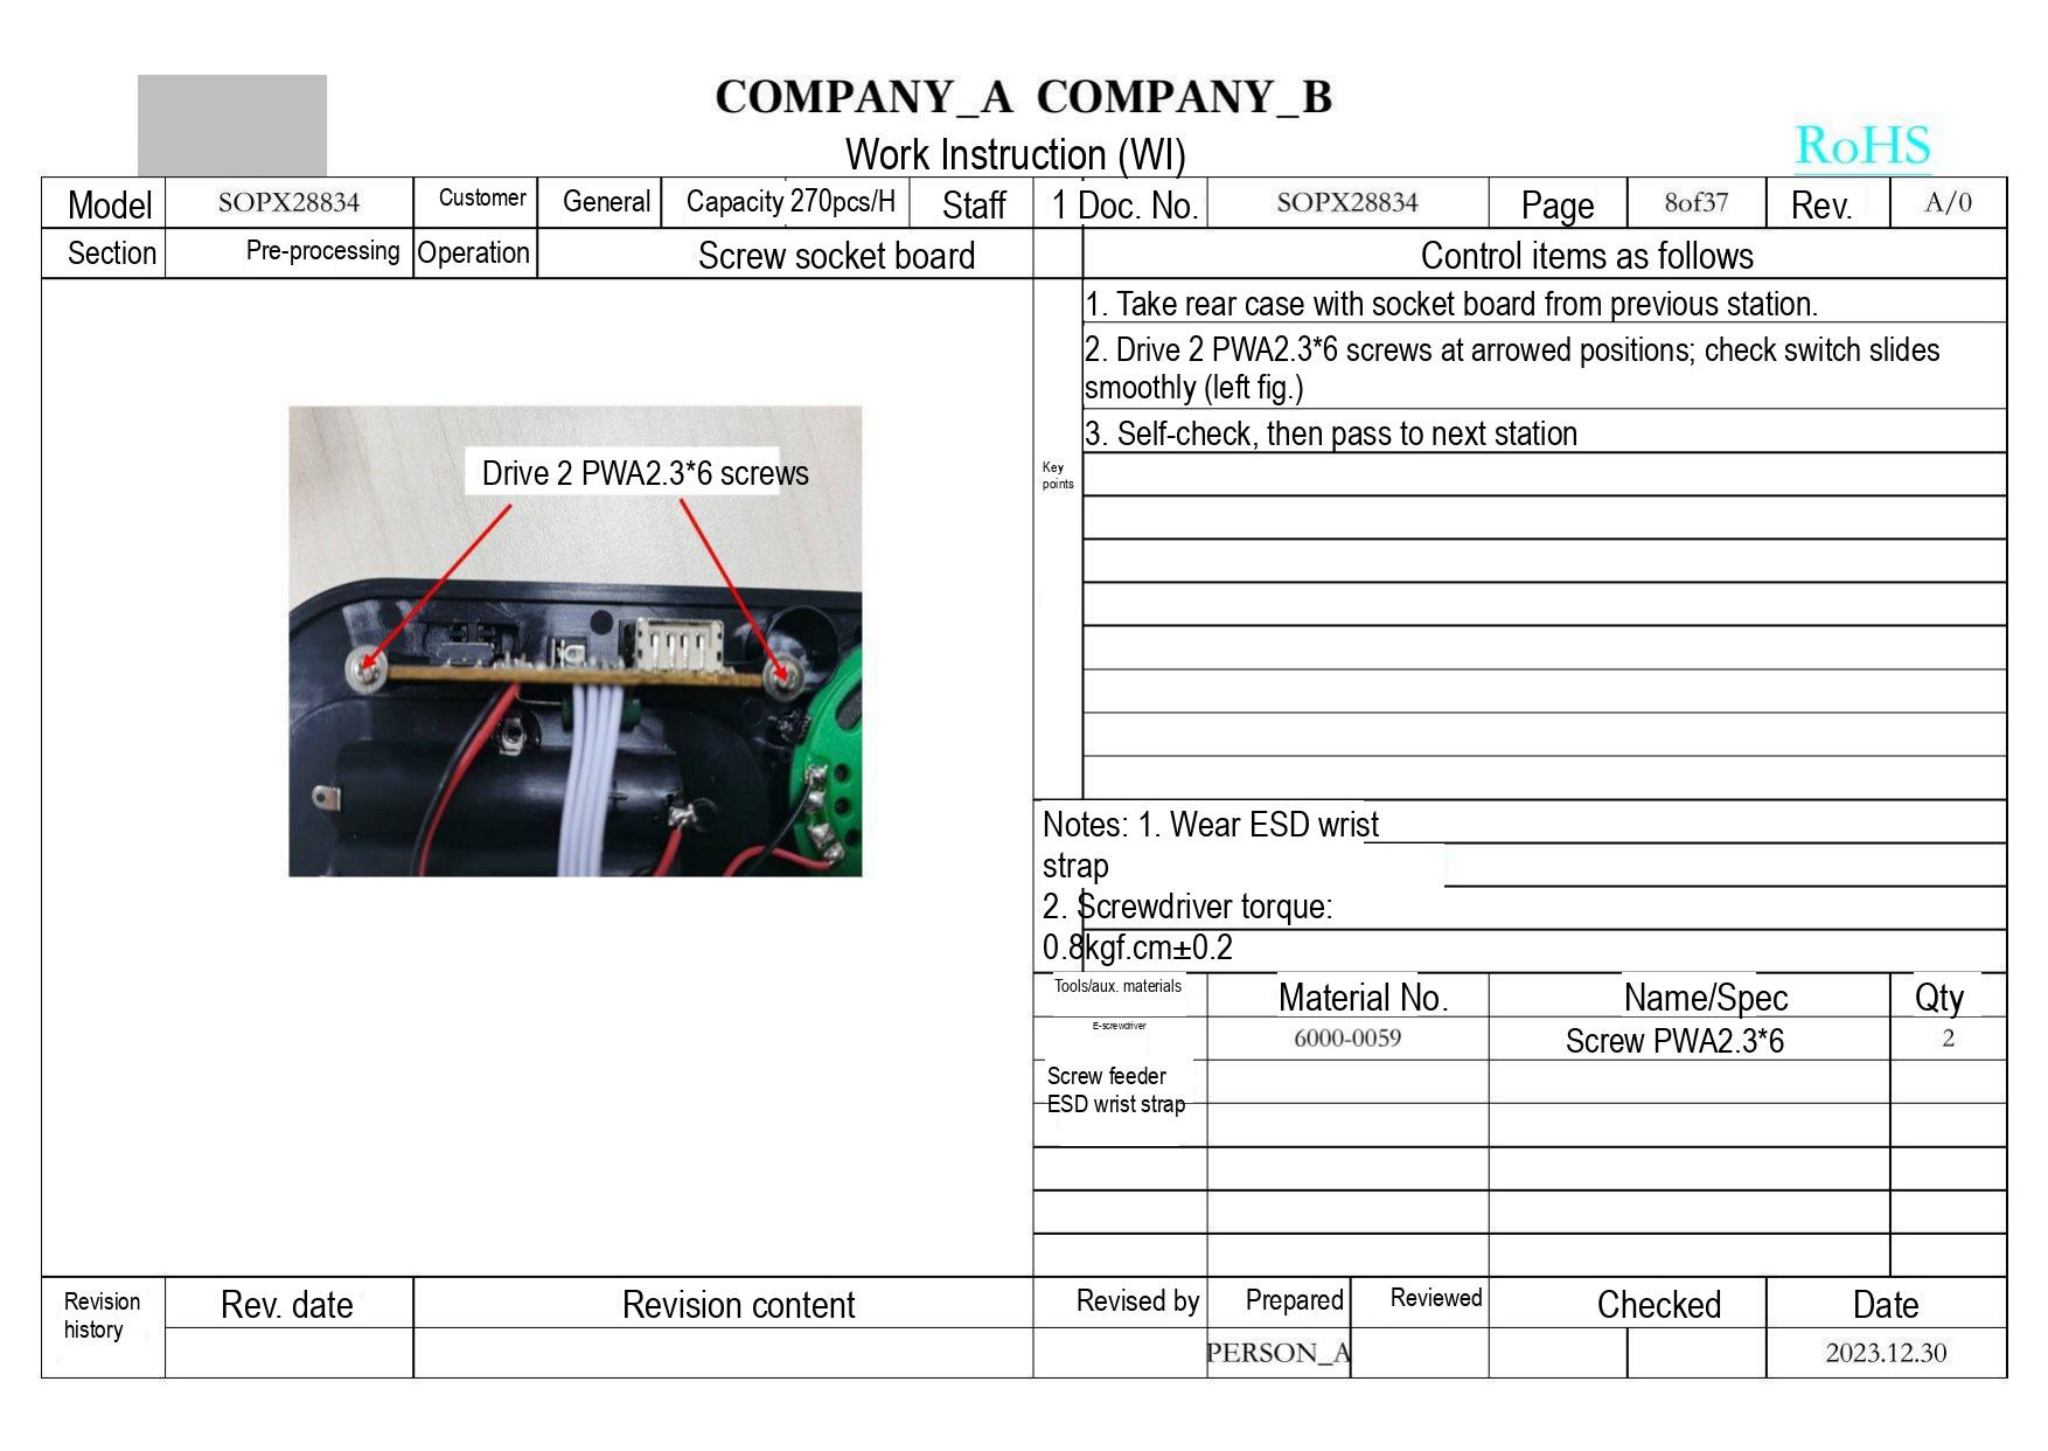COMPANY_A COMPANY_B
Work Instruction (WI)
RoHS

| Model | SOPX28834 | Customer | General | Capacity 270pcs/H | Staff | 1 Doc. No. | SOPX28834 | Page | 8of37 | Rev. | A/0 |
|---|---|---|---|---|---|---|---|---|---|---|---|
| Section | Pre-processing | Operation | Screw socket board | | | | | | | | |

Drive 2 PWA2.3*6 screws

| Key points | Control items as follows |
|---|---|
| | 1. Take rear case with socket board from previous station. |
| | 2. Drive 2 PWA2.3*6 screws at arrowed positions; check switch slides smoothly (left fig.) |
| | 3. Self-check, then pass to next station |

Notes: 1. Wear ESD wrist strap
2. Screwdriver torque: 0.8kgf.cm±0.2

| Tools/aux. materials | Material No. | Name/Spec | Qty |
|---|---|---|---|
| E-screwdriver<br>Screw feeder<br>ESD wrist strap | 6000-0059 | Screw PWA2.3*6 | 2 |

| Revision history | Rev. date | Revision content | Revised by | Prepared | Reviewed | Checked | Date |
|---|---|---|---|---|---|---|---|
| | | | | PERSON_A | | | 2023.12.30 |
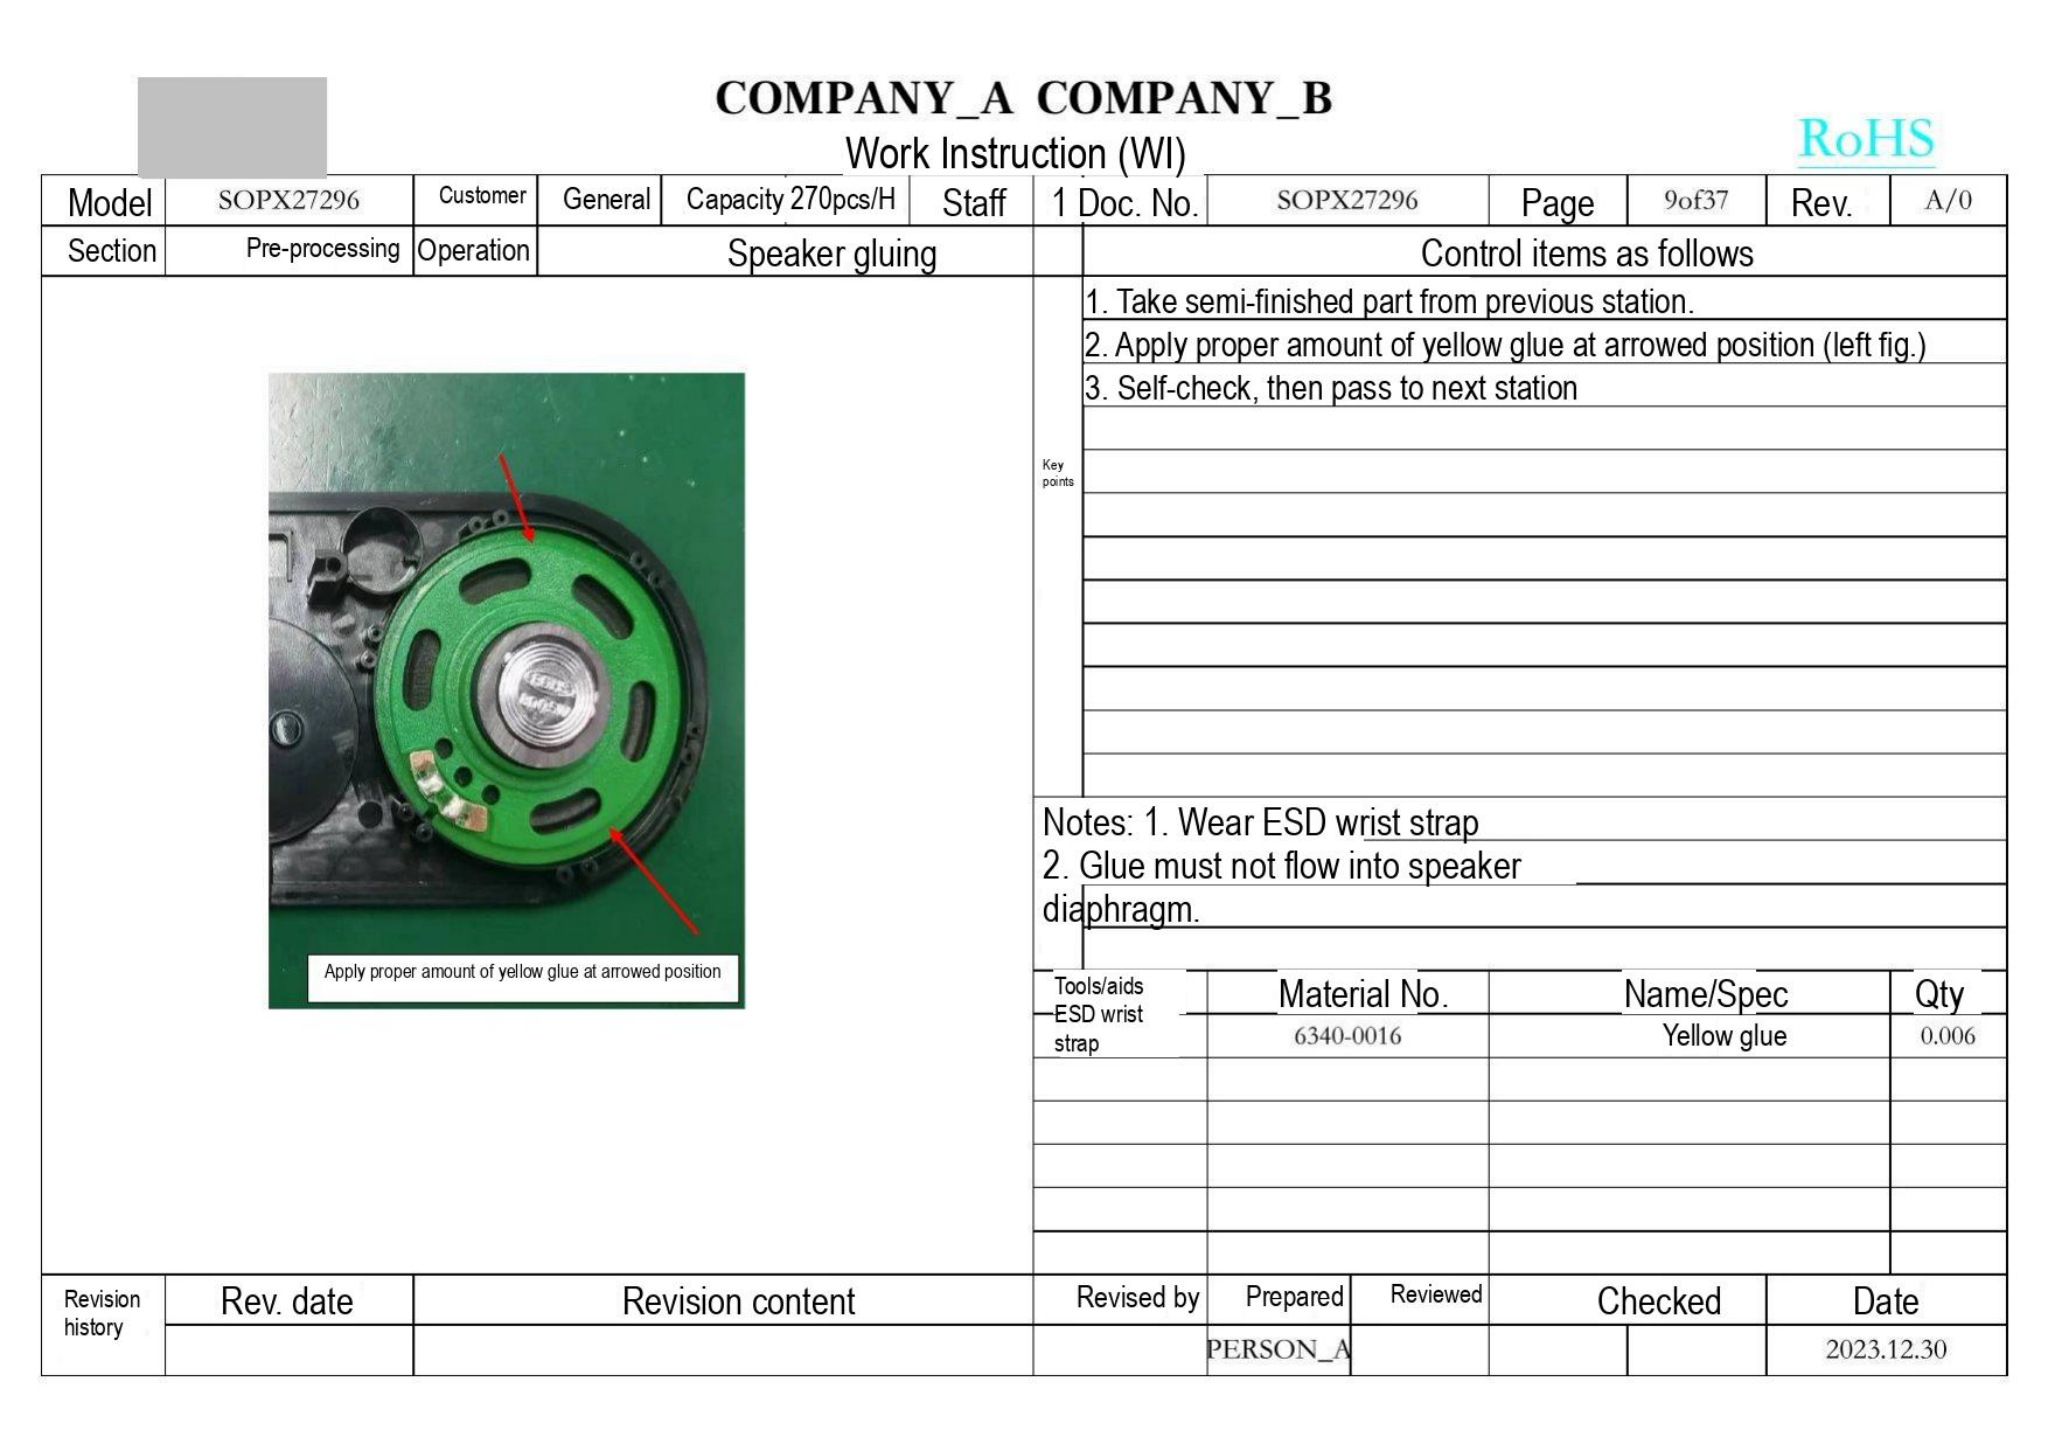COMPANY_A COMPANY_B
Work Instruction (WI)
RoHS

| Model | SOPX27296 | Customer | General | Capacity 270pcs/H | Staff | 1 | Doc. No. | SOPX27296 | Page | 9of37 | Rev. | A/0 |
|---|---|---|---|---|---|---|---|---|---|---|---|---|
| Section | Pre-processing | Operation | Speaker gluing | | | | | | | | | |

Control items as follows

Key points
1. Take semi-finished part from previous station.
2. Apply proper amount of yellow glue at arrowed position (left fig.)
3. Self-check, then pass to next station

Apply proper amount of yellow glue at arrowed position

Notes: 1. Wear ESD wrist strap
2. Glue must not flow into speaker diaphragm.

| Tools/aids | Material No. | Name/Spec | Qty |
|---|---|---|---|
| ESD wrist strap | 6340-0016 | Yellow glue | 0.006 |

| Revision history | Rev. date | Revision content | Revised by | Prepared | Reviewed | Checked | Date |
|---|---|---|---|---|---|---|---|
| | | | | PERSON_A | | | 2023.12.30 |
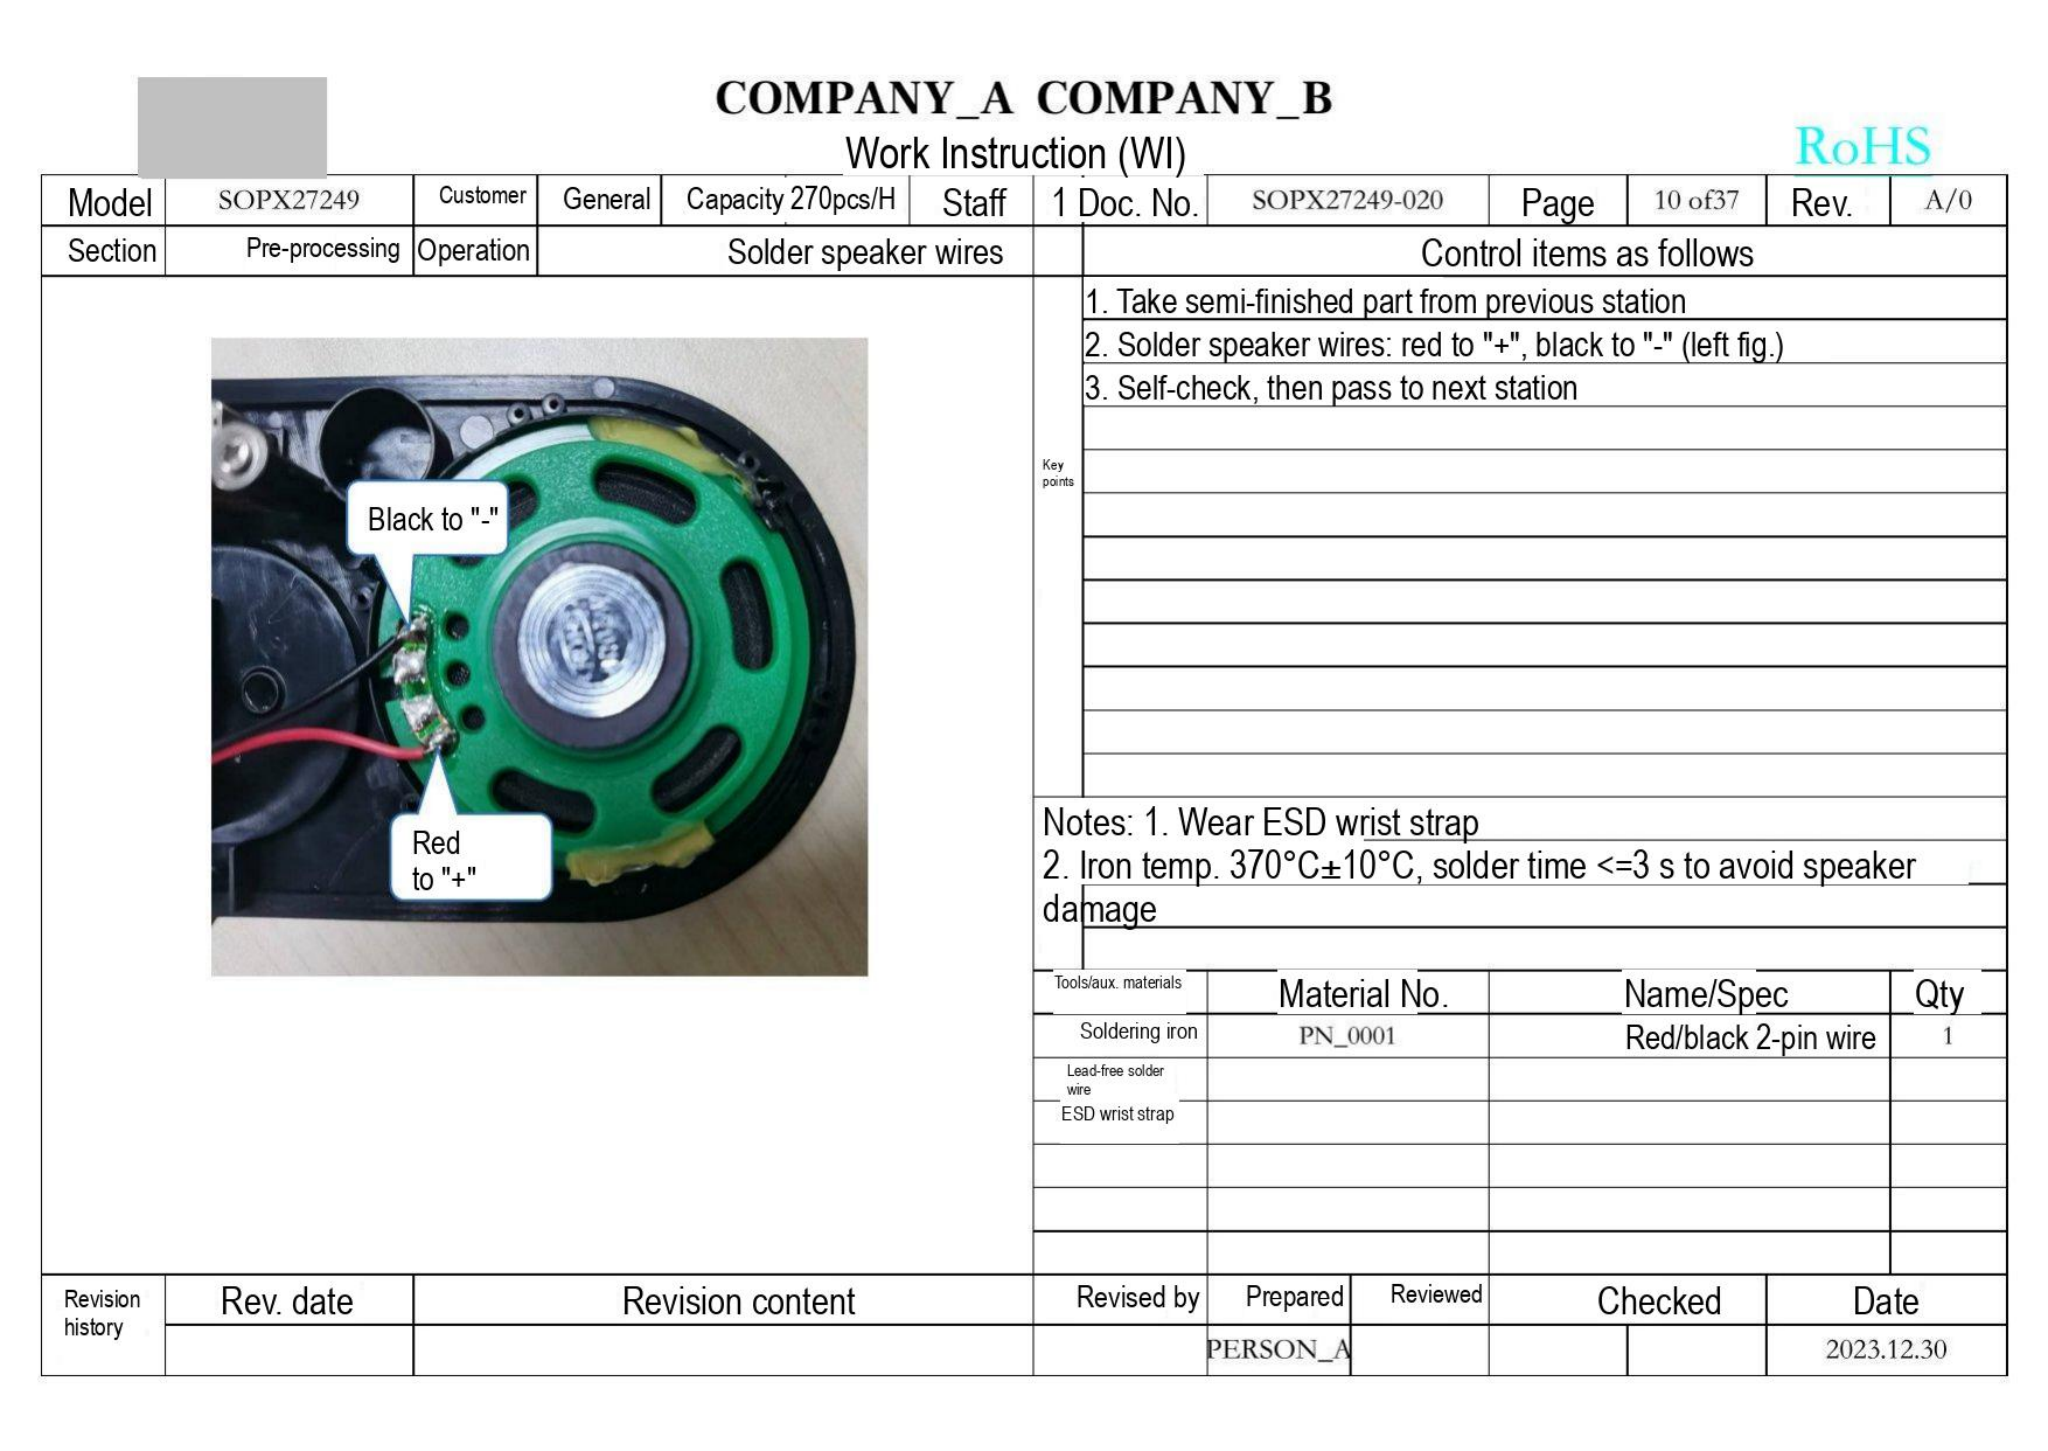COMPANY_A COMPANY_B
Work Instruction (WI)
RoHS

| Model | SOPX27249 | Customer | General | Capacity 270pcs/H | Staff | 1 Doc. No. | SOPX27249-020 | Page | 10 of37 | Rev. | A/0 |
|---|---|---|---|---|---|---|---|---|---|---|---|
| Section | Pre-processing | Operation | Solder speaker wires | | | | | | | | |

Black to "-"

Red to "+"

Control items as follows

Key points

1. Take semi-finished part from previous station
2. Solder speaker wires: red to "+", black to "-" (left fig.)
3. Self-check, then pass to next station

Notes: 1. Wear ESD wrist strap
2. Iron temp. 370°C±10°C, solder time <=3 s to avoid speaker damage

| Tools/aux. materials | Material No. | Name/Spec | Qty |
|---|---|---|---|
| Soldering iron | PN_0001 | Red/black 2-pin wire | 1 |
| Lead-free solder wire | | | |
| ESD wrist strap | | | |
| | | | |
| | | | |
| | | | |

| Revision history | Rev. date | Revision content | Revised by | Prepared | Reviewed | Checked | Date |
|---|---|---|---|---|---|---|---|
| | | | | PERSON_A | | | 2023.12.30 |
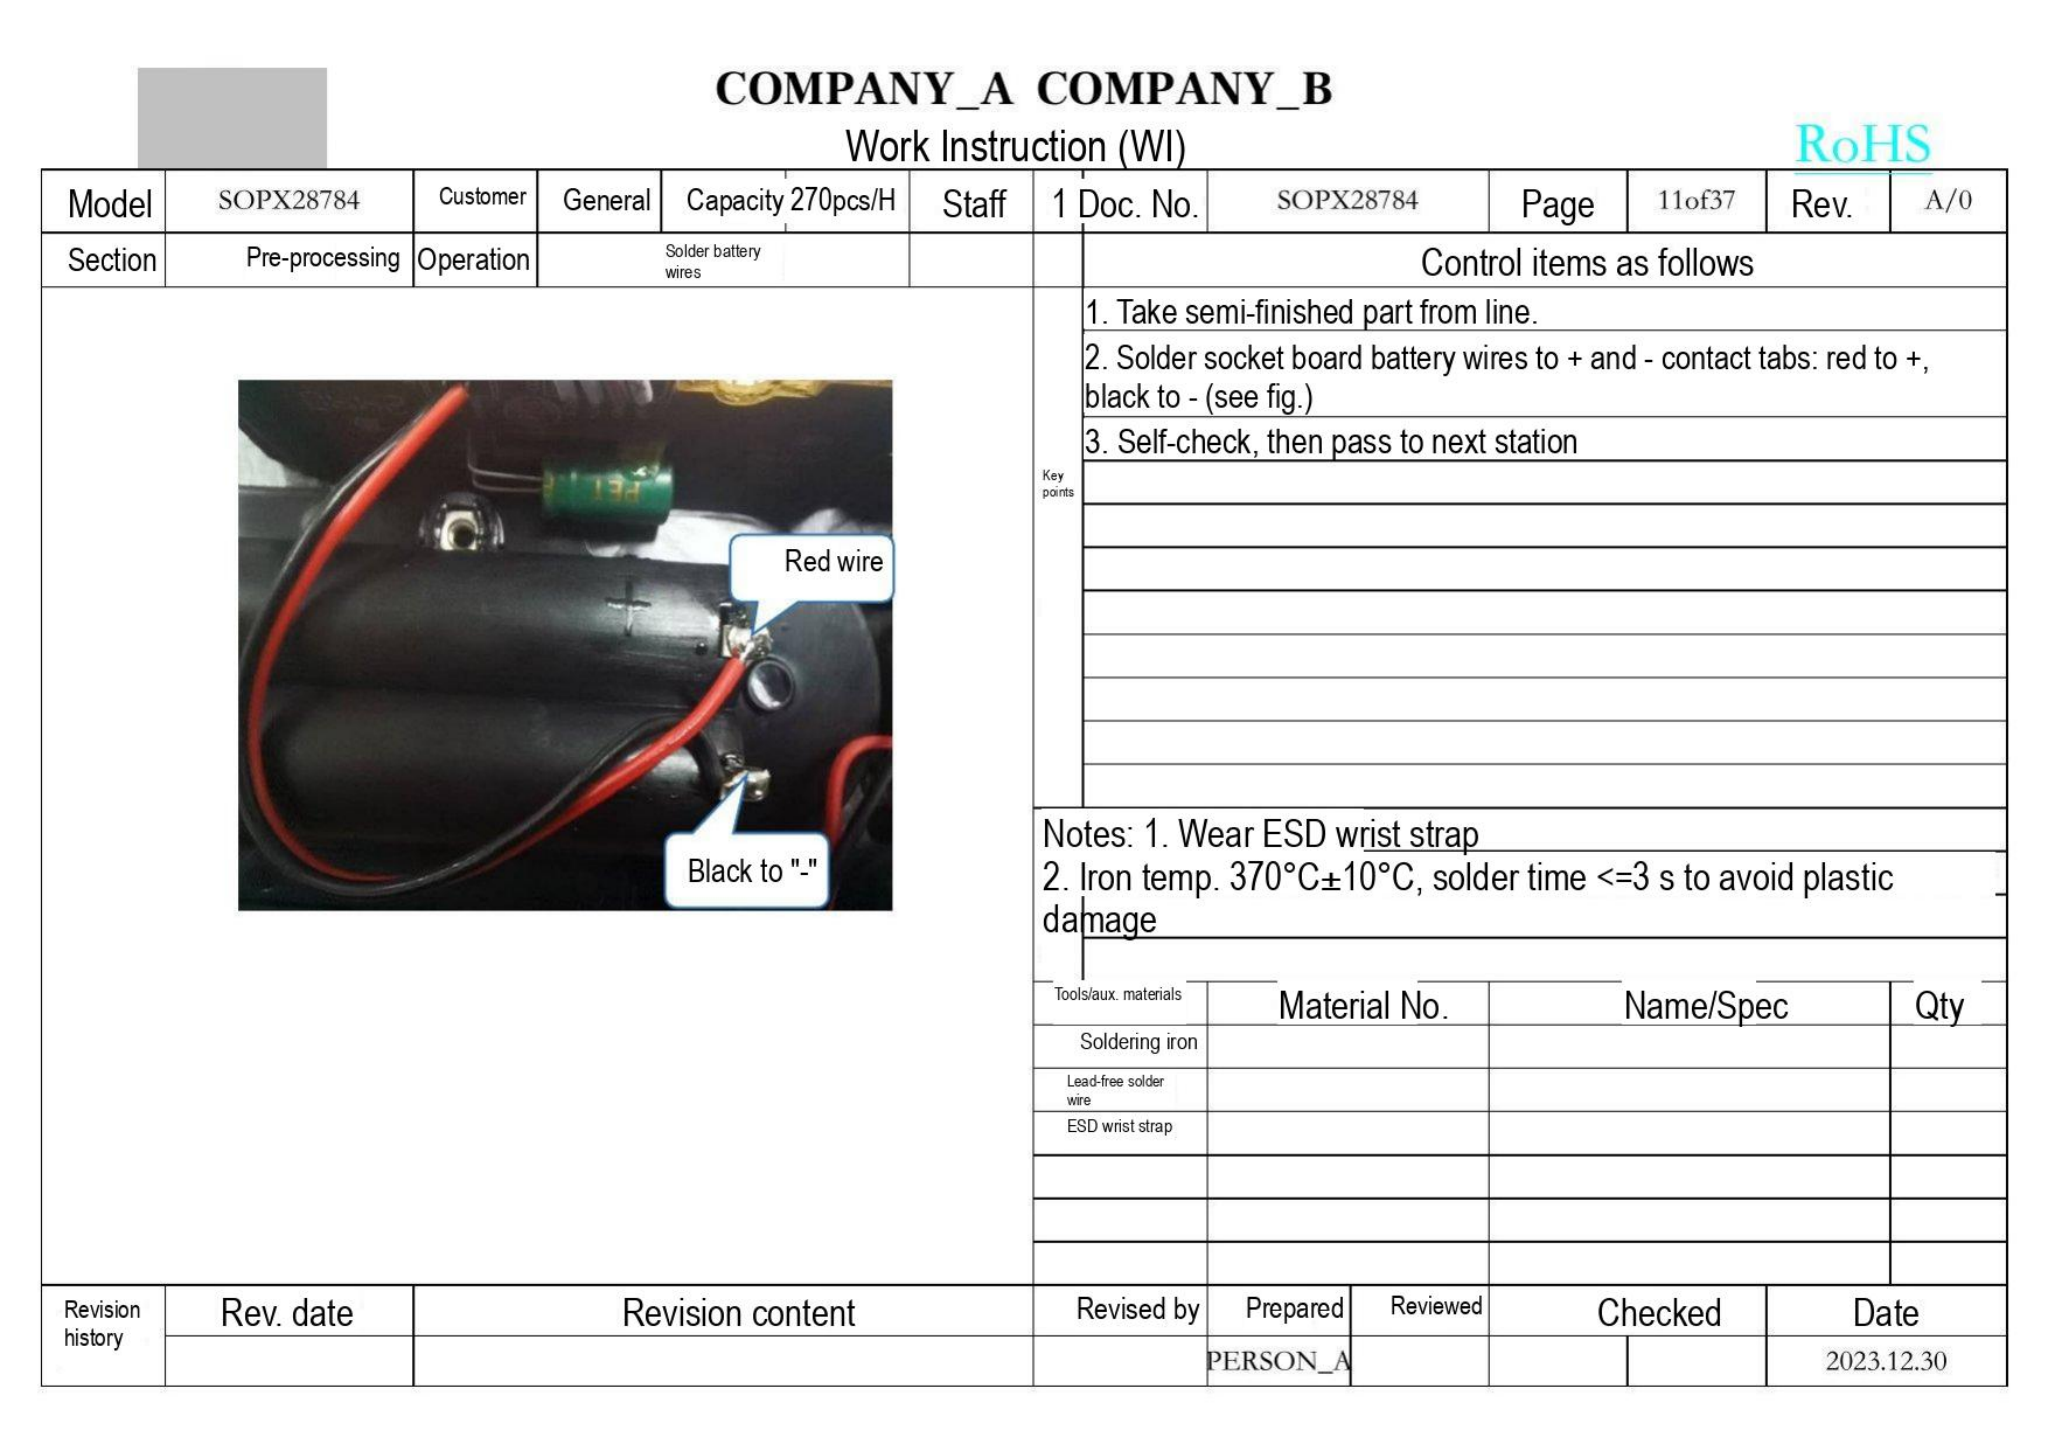COMPANY_A COMPANY_B
Work Instruction (WI)
RoHS

| Model | SOPX28784 | Customer | General | Capacity 270pcs/H | Staff | 1 | Doc. No. | SOPX28784 | Page | 11of37 | Rev. | A/0 |
|---|---|---|---|---|---|---|---|---|---|---|---|---|
| Section | Pre-processing | Operation | Solder battery wires | | | | | | | | | |

Control items as follows

Key points
1. Take semi-finished part from line.
2. Solder socket board battery wires to + and - contact tabs: red to +, black to - (see fig.)
3. Self-check, then pass to next station

Red wire
Black to "-"

Notes: 1. Wear ESD wrist strap
2. Iron temp. 370°C±10°C, solder time <=3 s to avoid plastic damage

| Tools/aux. materials | Material No. | Name/Spec | Qty |
|---|---|---|---|
| Soldering iron | | | |
| Lead-free solder wire | | | |
| ESD wrist strap | | | |
| | | | |
| | | | |
| | | | |

| Revision history | Rev. date | Revision content | Revised by | Prepared | Reviewed | Checked | Date |
|---|---|---|---|---|---|---|---|
| | | | | PERSON_A | | | 2023.12.30 |
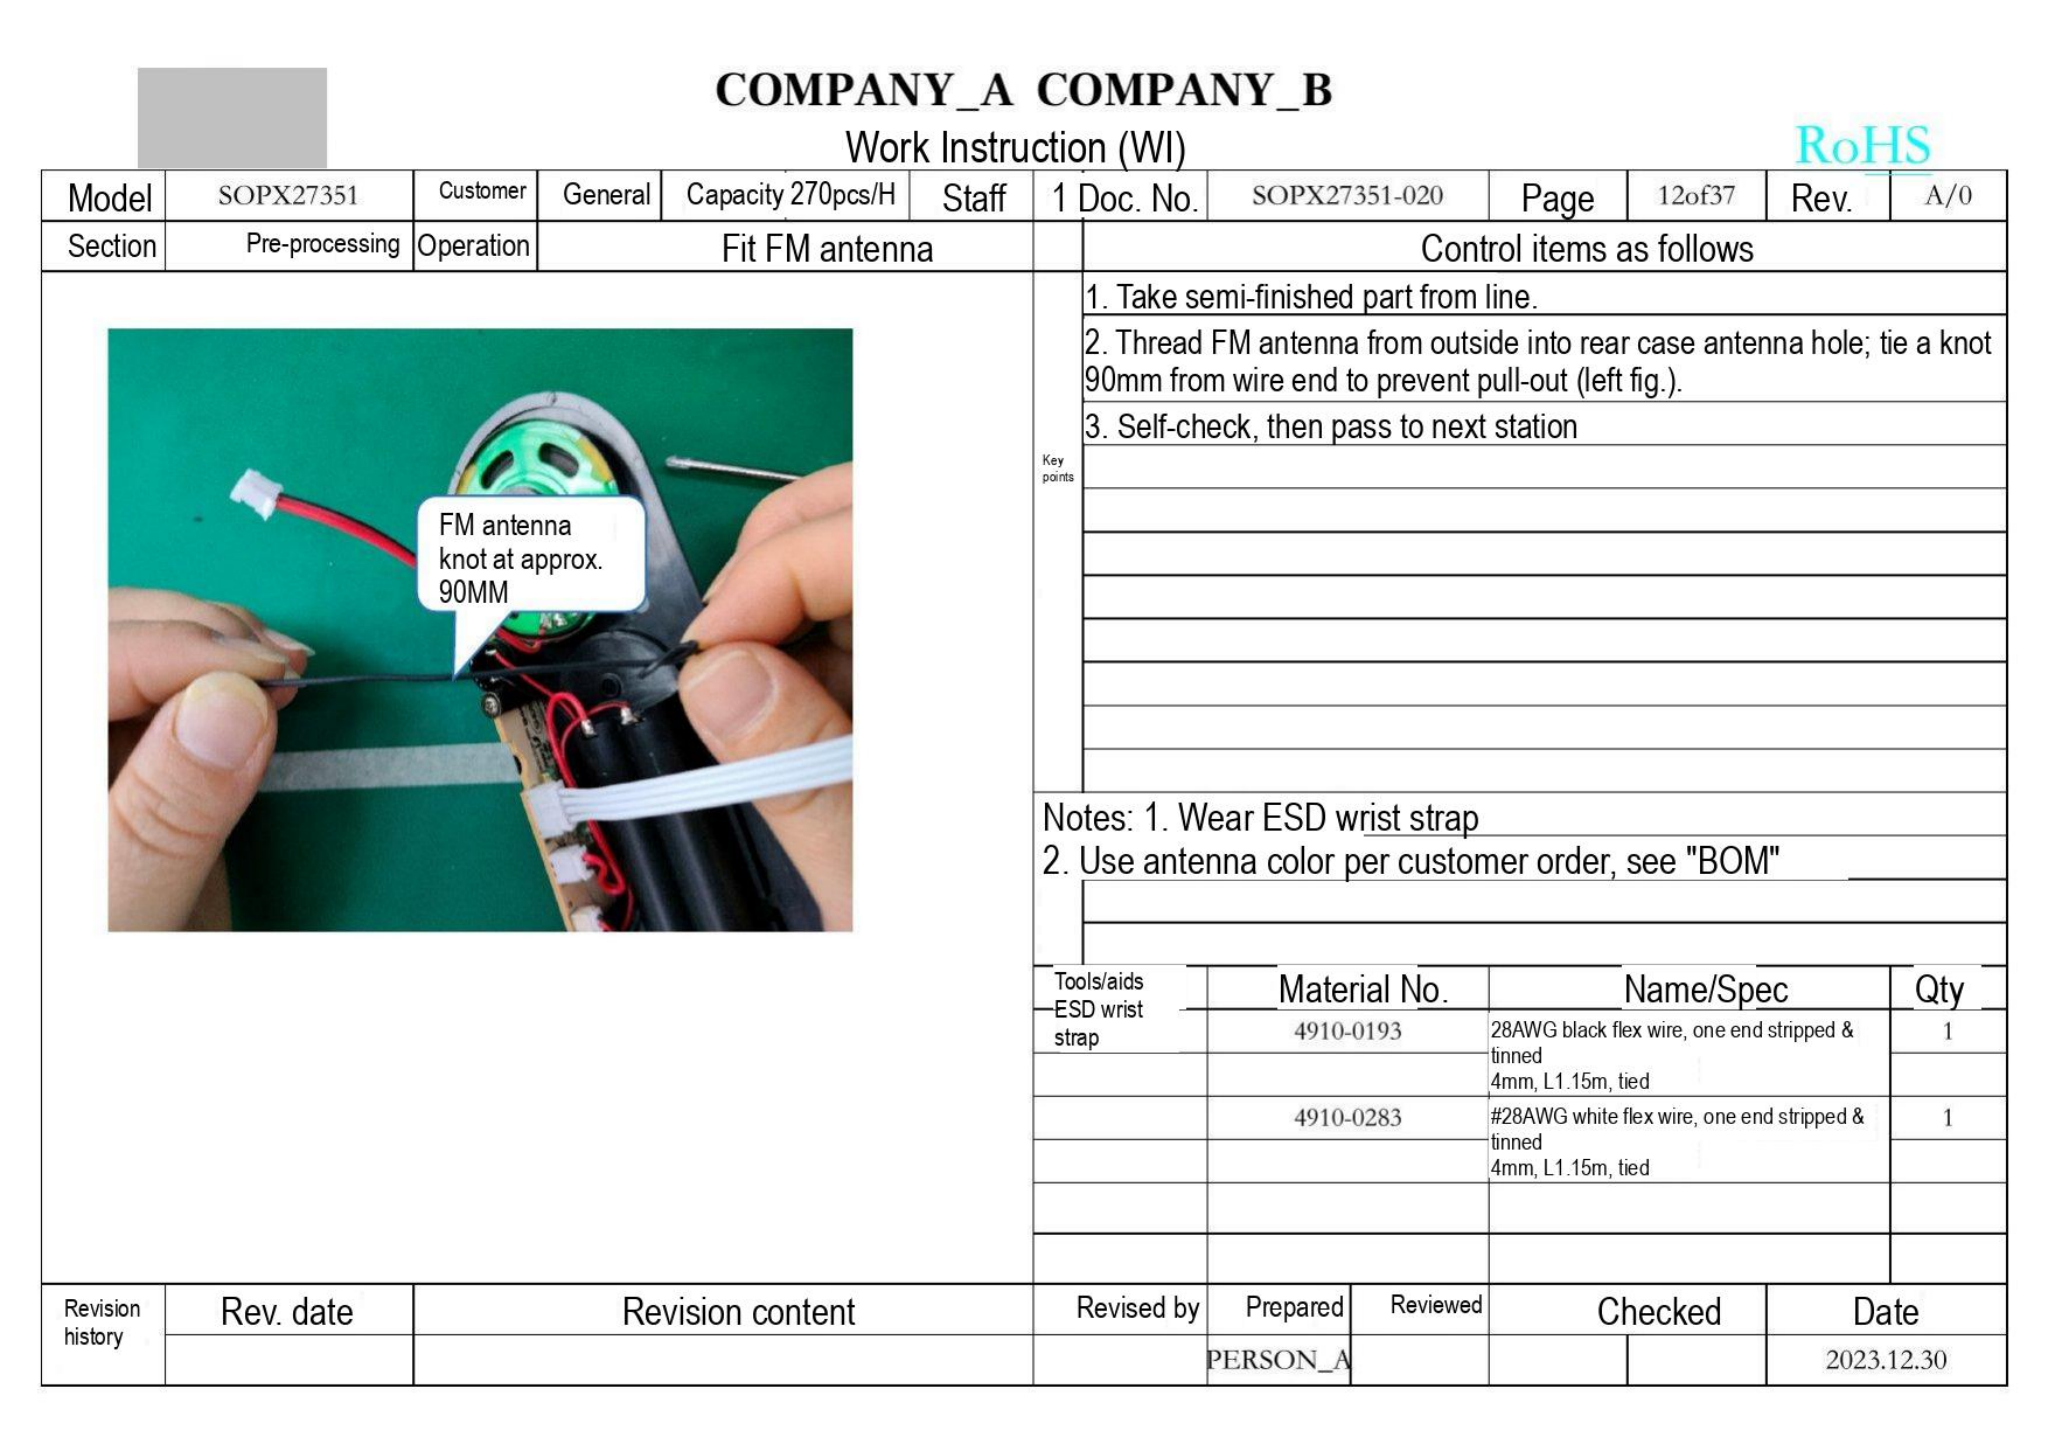COMPANY_A COMPANY_B

Work Instruction (WI)

RoHS

| Model | SOPX27351 | Customer | General | Capacity 270pcs/H | Staff | 1 Doc. No. | SOPX27351-020 | Page | 12of37 | Rev. | A/0 |
|---|---|---|---|---|---|---|---|---|---|---|---|
| Section | Pre-processing | Operation | Fit FM antenna | | | Control items as follows | | | | | |

FM antenna knot at approx. 90MM

Key points

1. Take semi-finished part from line.
2. Thread FM antenna from outside into rear case antenna hole; tie a knot 90mm from wire end to prevent pull-out (left fig.).
3. Self-check, then pass to next station

Notes: 1. Wear ESD wrist strap
2. Use antenna color per customer order, see "BOM"

| Tools/aids | Material No. | Name/Spec | Qty |
|---|---|---|---|
| ESD wrist strap | 4910-0193 | 28AWG black flex wire, one end stripped & tinned 4mm, L1.15m, tied | 1 |
| | 4910-0283 | #28AWG white flex wire, one end stripped & tinned 4mm, L1.15m, tied | 1 |

| Revision history | Rev. date | Revision content | Revised by | Prepared | Reviewed | Checked | Date |
|---|---|---|---|---|---|---|---|
| | | | | PERSON_A | | | 2023.12.30 |
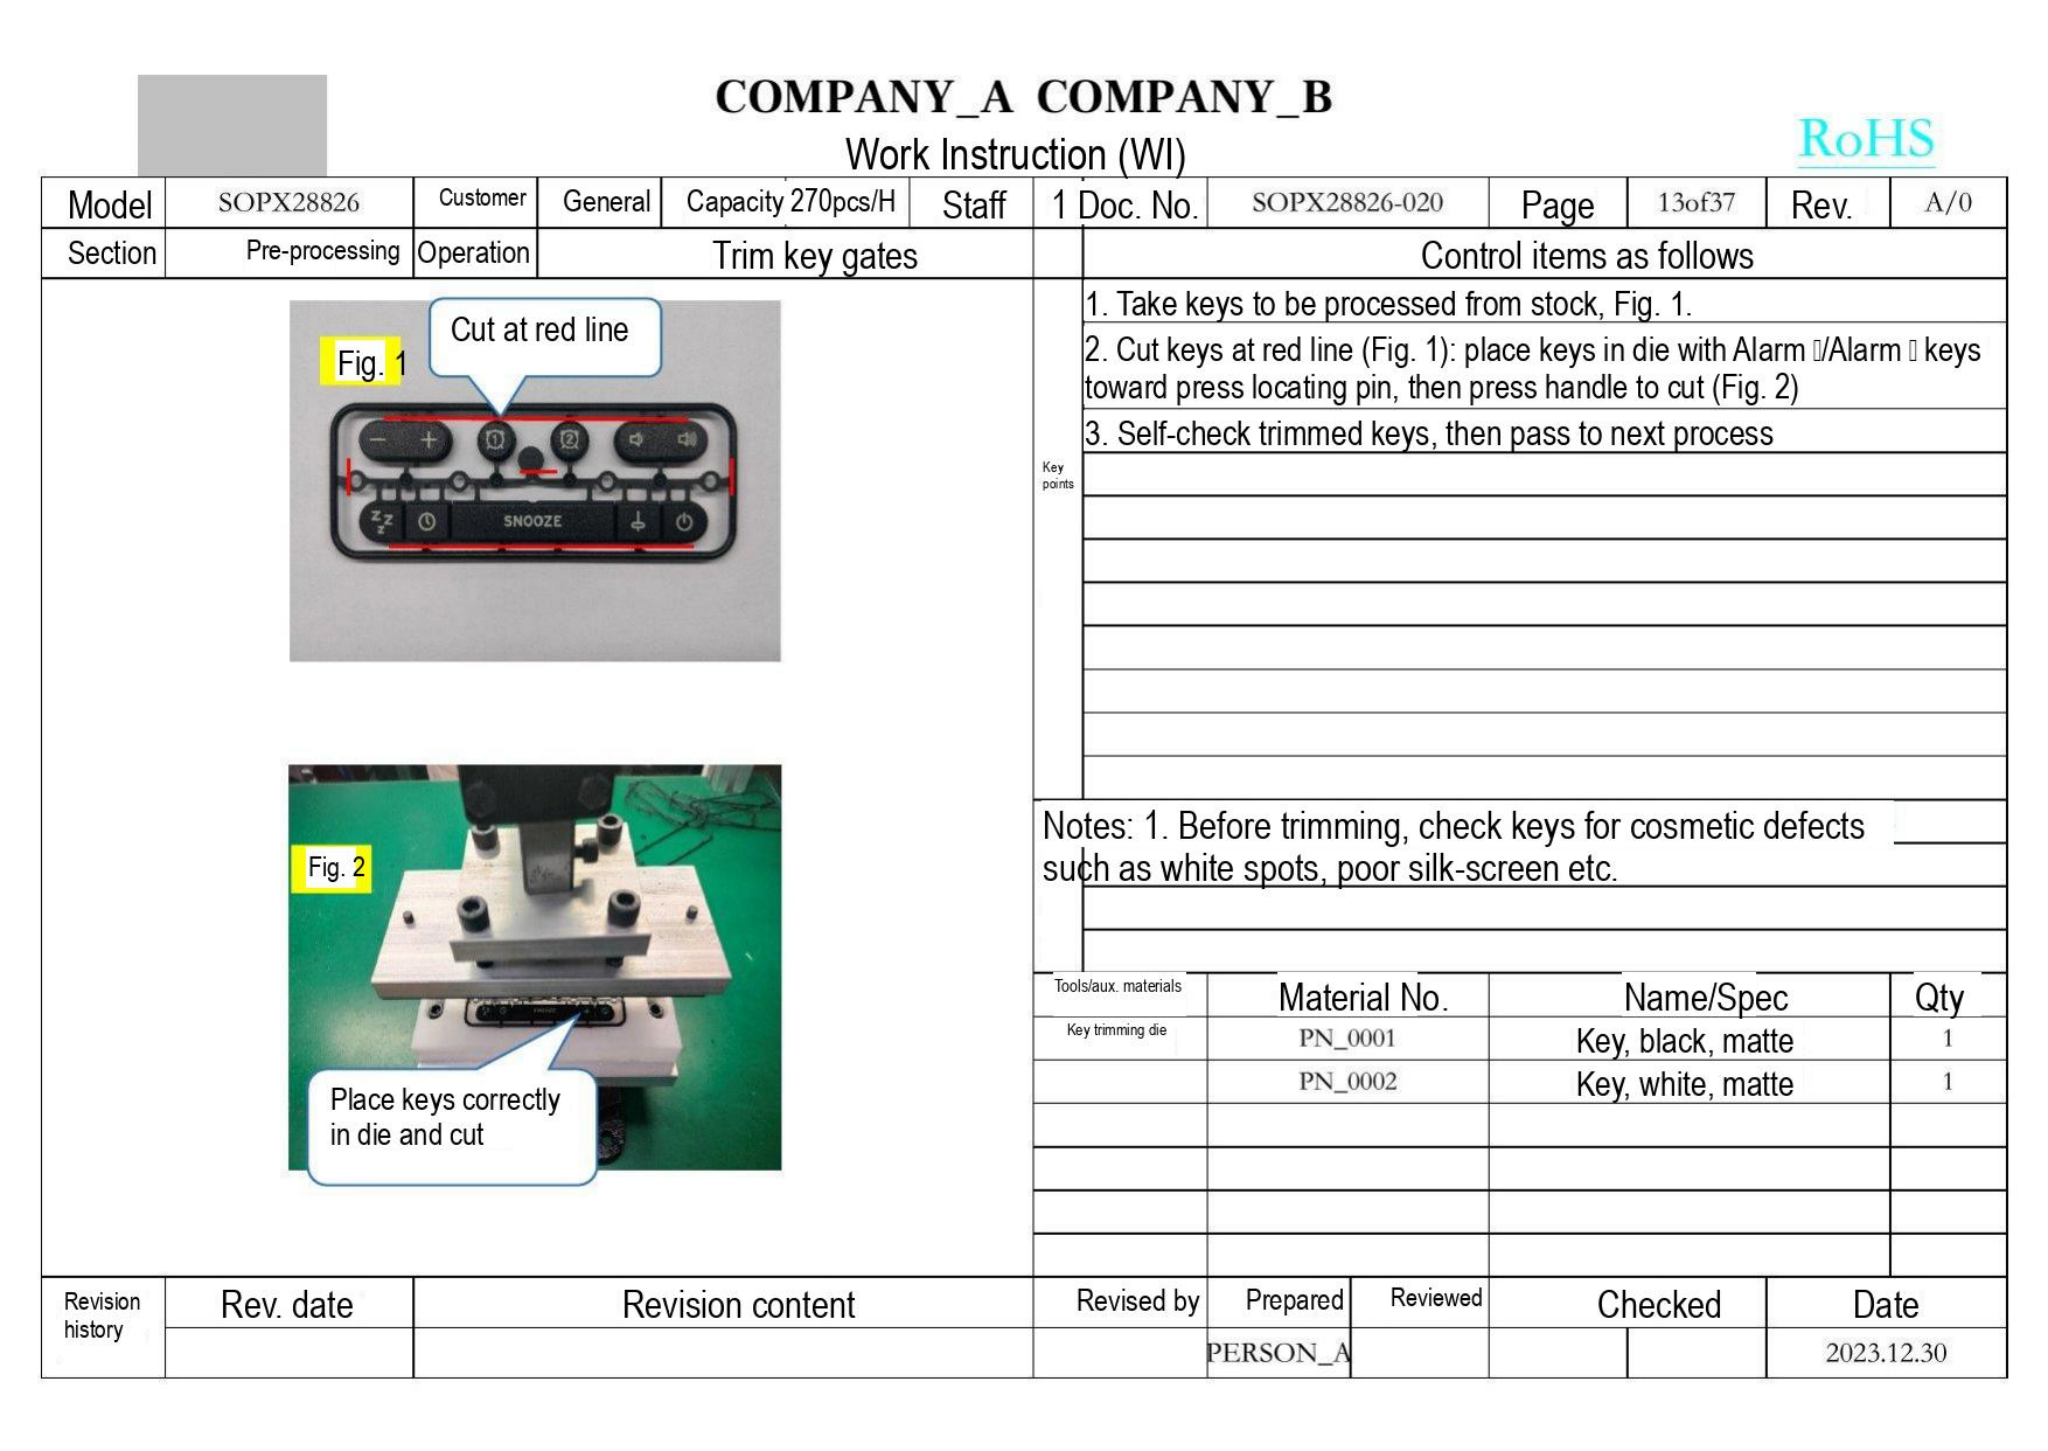COMPANY_A COMPANY_B

Work Instruction (WI)

RoHS

| Model | SOPX28826 | Customer | General | Capacity 270pcs/H | Staff | 1 | Doc. No. | SOPX28826-020 | Page | 13of37 | Rev. | A/0 |
|---|---|---|---|---|---|---|---|---|---|---|---|---|
| Section | Pre-processing | Operation | Trim key gates | | | | Control items as follows | | | | | |

Fig. 1

Cut at red line

SNOOZE

Fig. 2

Place keys correctly in die and cut

| Key points | Control items as follows |
|---|---|
| | 1. Take keys to be processed from stock, Fig. 1. |
| | 2. Cut keys at red line (Fig. 1): place keys in die with Alarm ▯/Alarm ▯ keys toward press locating pin, then press handle to cut (Fig. 2) |
| | 3. Self-check trimmed keys, then pass to next process |

Notes: 1. Before trimming, check keys for cosmetic defects such as white spots, poor silk-screen etc.

| Tools/aux. materials | Material No. | Name/Spec | Qty |
|---|---|---|---|
| Key trimming die | PN_0001 | Key, black, matte | 1 |
| | PN_0002 | Key, white, matte | 1 |

| Revision history | Rev. date | Revision content | Revised by | Prepared | Reviewed | Checked | Date |
|---|---|---|---|---|---|---|---|
| | | | | PERSON_A | | | 2023.12.30 |
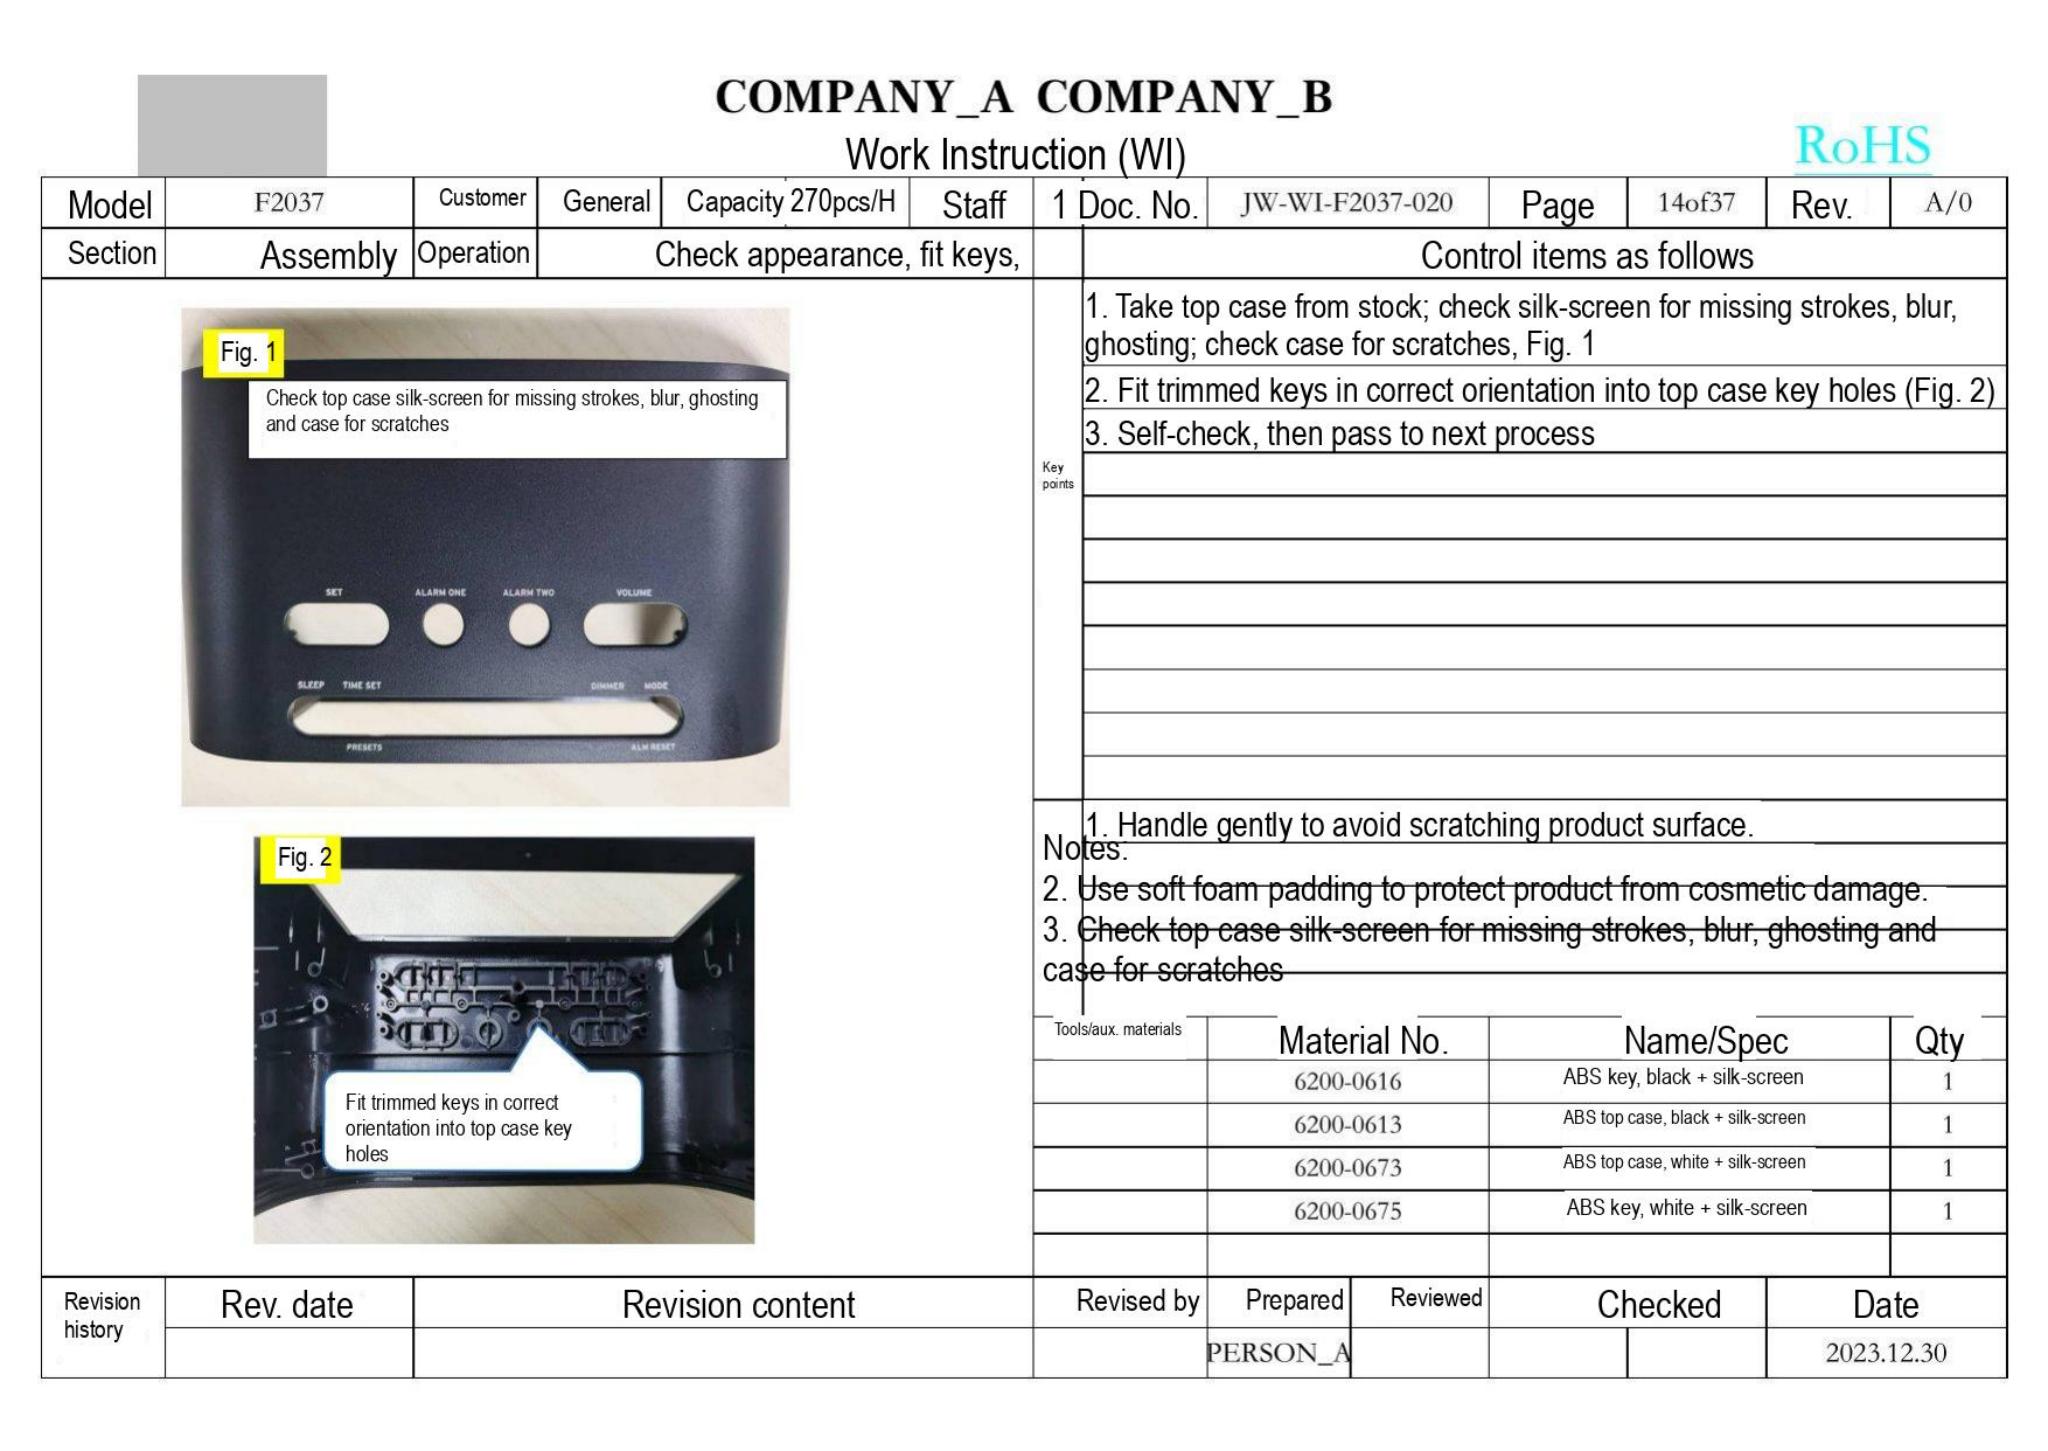# COMPANY_A COMPANY_B

Work Instruction (WI)

RoHS

| Model | F2037 | Customer | General | Capacity 270pcs/H | Staff | 1 | Doc. No. | JW-WI-F2037-020 | Page | 14of37 | Rev. | A/0 |
|---|---|---|---|---|---|---|---|---|---|---|---|---|
| Section | Assembly | Operation | Check appearance, fit keys, | | | | | | | | | |

Fig. 1

Check top case silk-screen for missing strokes, blur, ghosting and case for scratches

SET ALARM ONE ALARM TWO VOLUME

SLEEP TIME SET DIMMER MODE

PRESETS ALM RESET

Fig. 2

Fit trimmed keys in correct orientation into top case key holes

Control items as follows

Key points

1. Take top case from stock; check silk-screen for missing strokes, blur, ghosting; check case for scratches, Fig. 1
2. Fit trimmed keys in correct orientation into top case key holes (Fig. 2)
3. Self-check, then pass to next process

Notes:
1. Handle gently to avoid scratching product surface.
2. ~~Use soft foam padding to protect product from cosmetic damage.~~
3. ~~Check top case silk-screen for missing strokes, blur, ghosting and case for scratches~~

| Tools/aux. materials | Material No. | Name/Spec | Qty |
|---|---|---|---|
| | 6200-0616 | ABS key, black + silk-screen | 1 |
| | 6200-0613 | ABS top case, black + silk-screen | 1 |
| | 6200-0673 | ABS top case, white + silk-screen | 1 |
| | 6200-0675 | ABS key, white + silk-screen | 1 |
| | | | |

| Revision history | Rev. date | Revision content | Revised by | Prepared | Reviewed | Checked | Date |
|---|---|---|---|---|---|---|---|
| | | | | PERSON_A | | | 2023.12.30 |